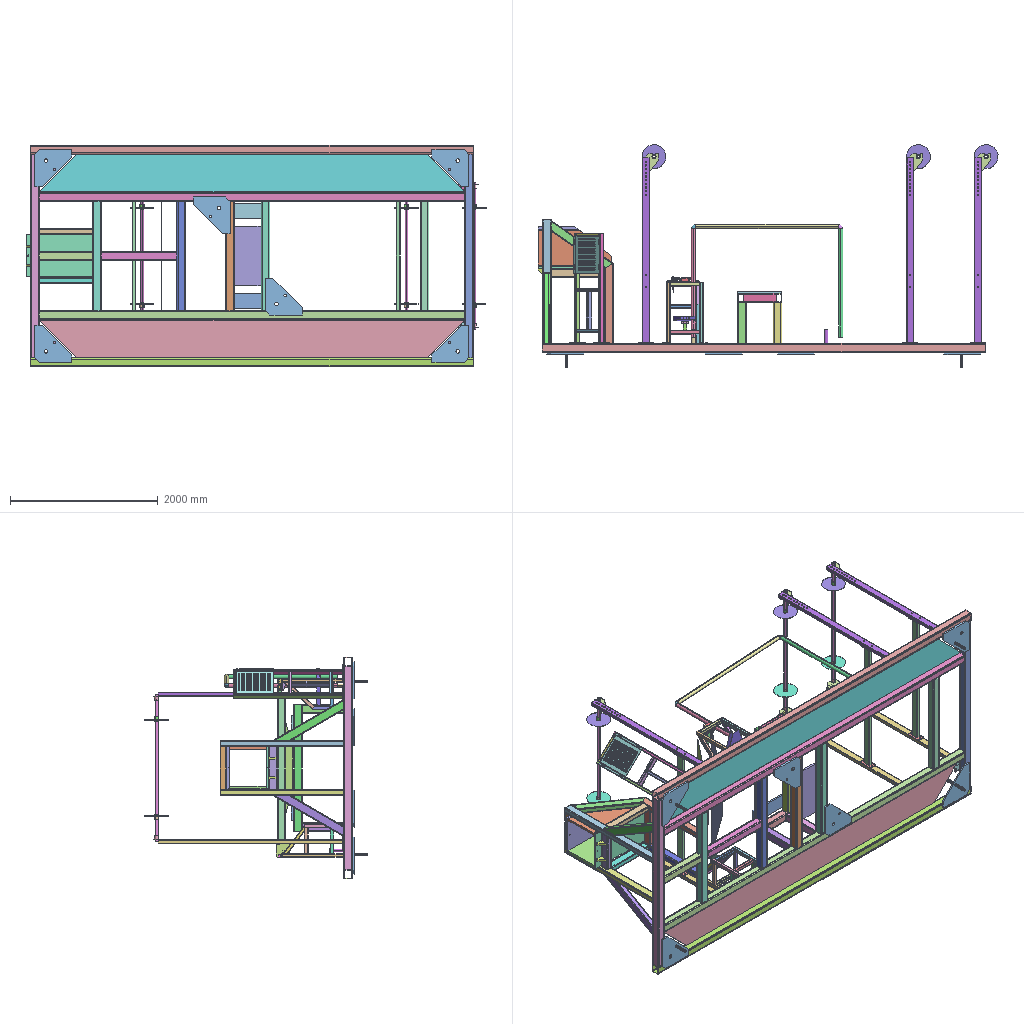Assembly | SolidWorks | 56 different items | 111 placed | box 6232 x 3016 x 3000 mm
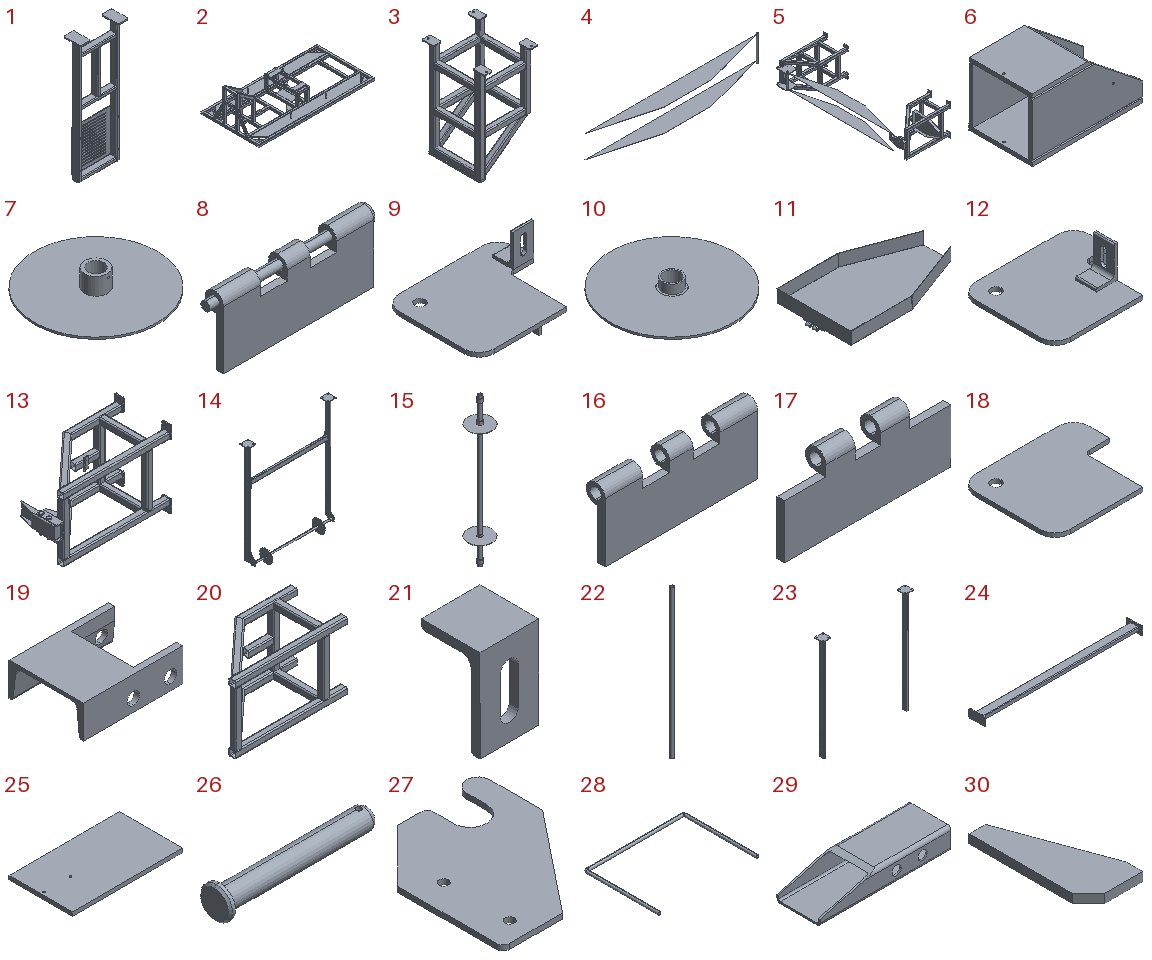Parts list (item | name | quantity | parent item | size | volume | features):
1 | (subassembly) | x1 | - | 580 x 200 x 1494 mm | 6577657 mm3 | -
2 | (subassembly) | x1 | - | 6060 x 3000 x 1995 mm | 369969133 mm3 | features ReferencePattern 10, MirrorCompFeat 5, CompositeCurve 1
3 | (subassembly) | x1 | in 5 | 470 x 550 x 847 mm | 5189358 mm3 | features ReferencePattern 3, MirrorCompFeat 2
4 | (subassembly) | x1 | in 5 | 2055 x 200.072 x 310 mm | 659869 mm3 | -
5 | (subassembly) | x1 | - | 917 x 2571 x 600 mm | 11540187 mm3 | features MirrorCompFeat 1, ReferencePattern 1
6 | (subassembly) | x1 | - | 1000 x 570 x 570 mm | 59141970 mm3 | -
7 | (subassembly) | x3 | in 15 | 325 x 325 x 74 mm | 481042 mm3 | -
8 | (subassembly) | x1 | in 13 | 92 x 10.5 x 38.25 mm | 14844 mm3 | -
9 | (subassembly) | x1 | in 5 | 220 x 184 x 134 mm | 313255 mm3 | -
10 | (subassembly) | x3 | in 15 | 325 x 325 x 74 mm | 481042 mm3 | -
11 | (subassembly) | x1 | in 5 | 510.75 x 300 x 60.5 mm | 296011 mm3 | -
12 | (subassembly) | x1 | in 5 | 220 x 184 x 134 mm | 313255 mm3 | -
13 | (subassembly) | x1 | in 5 | 891 x 440 x 600 mm | 4747445 mm3 | features ReferencePattern 3, MirrorCompFeat 2
14 | (subassembly) | x3 | - | 2200 x 372.5 x 2697 mm | 11177165 mm3 | -
15 | (subassembly) | x3 | in 14 | 325 x 325 x 2000 mm | 1601927 mm3 | features ReferencePattern 2, MirrorCompFeat 1
16 | - | x1 | in 8 | 85 x 10.5 x 38.25 mm | 12934 mm3 | features ICE 2, Chamfer 1, Cut 1, Extrusion 1
17 | - | x1 | in 11 | 85 x 10.5 x 38.25 mm | 11305 mm3 | features ICE 2, Chamfer 1, Cut 1, Extrusion 1
18 | - | x1 | in 12 | 220 x 184 x 8 mm | 271263 mm3 | features Extrusion 1
19 | - | x1 | in 13 | 160 x 120 x 53 mm | 192954 mm3 | features ICE 2, 3DProfileFeature 1, WeldMemberFeat 1, WeldmentFeature 1
20 | - | x1 | in 13 | 825 x 420 x 500 mm | 3812160 mm3 | features WeldCornerFeat 3, WeldMemberFeat 2, 3DProfileFeature 1, Cut 1, WeldmentFeature 1
21 | - | x3 | in 5, 12 | 40 x 40 x 63 mm | 20996 mm3 | features 3DProfileFeature 1, Cut 1, WeldMemberFeat 1, WeldmentFeature 1
22 | - | x3 | in 15 | 42 x 42 x 2000 mm | 502655 mm3 | features Extrusion 1
23 | - | x3 | in 14 | 2200 x 200 x 2514 mm | 6513642 mm3 | features HoleWzd 4, Fillet 2, ICE 2, MirrorSolid 2, 3DProfileFeature 1, LPattern 1, WeldMemberFeat 1, WeldmentFeature 1
24 | - | x3 | in 14 | 1950 x 200 x 100 mm | 2501619 mm3 | features Fillet 1, HoleWzd 1, ICE 1, MirrorSolid 1, WeldMemberFeat 1, WeldmentFeature 1
25 | - | x1 | in 6 | 1000 x 570 x 35 mm | 19933163 mm3 | features 3DProfileFeature 1, Extrusion 1, HoleWzd 1
26 | - | x2 | in 13 | 145 x 30 x 30 mm | 46693 mm3 | features Chamfer 1, Fillet 1, ICE 1, Revolution 1
27 | - | x6 | in 14 | 210 x 247.5 x 8 mm | 279988 mm3 | features Extrusion 1
28 | - | x1 | - | 2060 x 1530 x 60 mm | 4297442 mm3 | features 3DProfileFeature 1, WeldMemberFeat 1, WeldmentFeature 1
29 | - | x1 | in 13 | 300 x 100 x 50 mm | 358178 mm3 | features ICE 2, 3DProfileFeature 1, WeldMemberFeat 1, WeldmentFeature 1
30 | - | x2 | in 13 | 50 x 110 x 8 mm | 29800 mm3 | features Chamfer 1, Extrusion 1
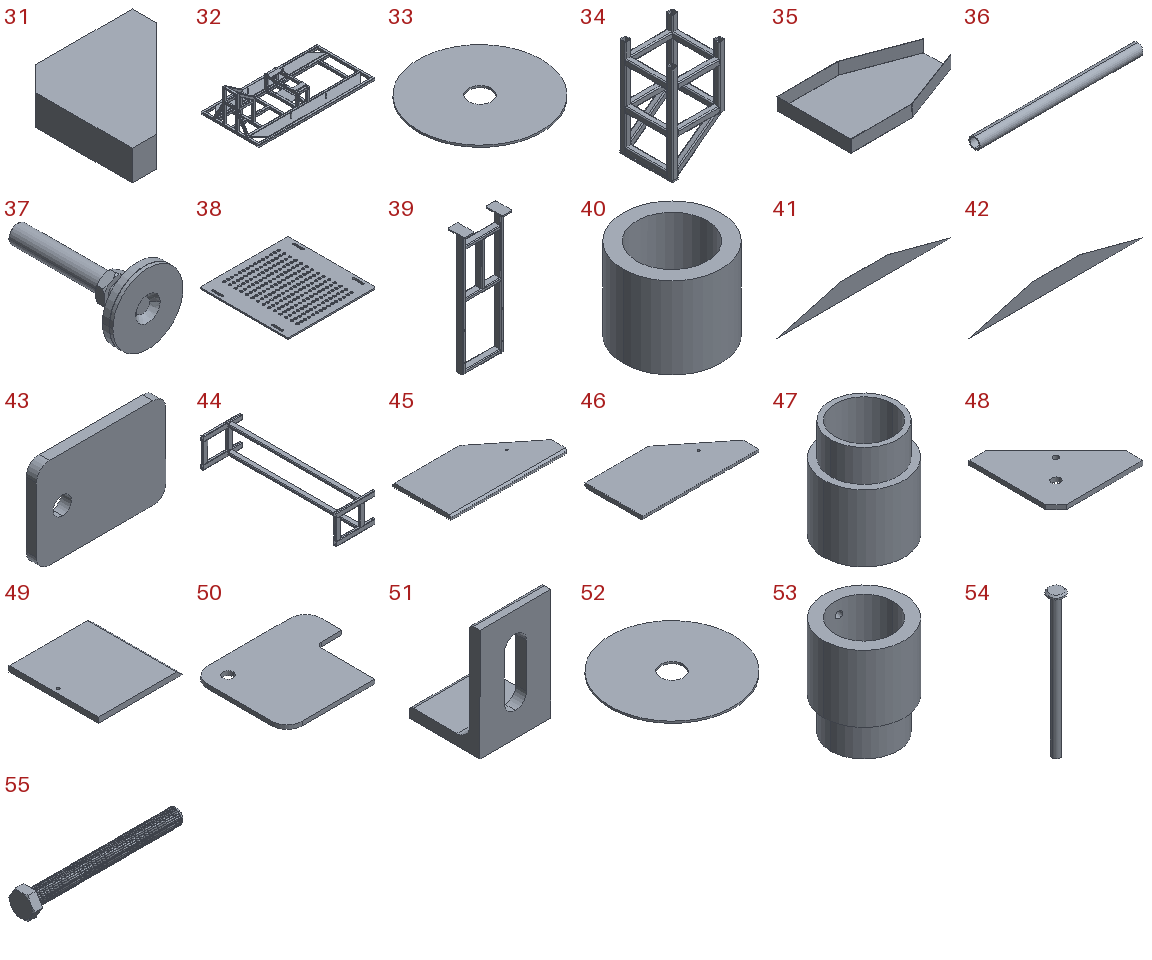31 | - | x2 | in 2 | 100 x 100 x 25 mm | 165000 mm3 | features Extrusion 1
32 | - | x1 | in 2 | 6000 x 3000 x 1795 mm | 349583429 mm3 | features WeldCornerFeat 9, ICE 4, MoveCopyBody 4, WeldMemberFeat 3, MirrorSolid 2, 3DProfileFeature 1, LPattern 1, WeldmentFeature 1
33 | - | x3 | in 7 | 325 x 325 x 5 mm | 400176 mm3 | features Extrusion 1
34 | - | x1 | in 3 | 450 x 450 x 839 mm | 4973031 mm3 | features WeldCornerFeat 2, WeldMemberFeat 2, 3DProfileFeature 1, ICE 1, WeldmentFeature 1
35 | - | x1 | in 11 | 500 x 300 x 50 mm | 284706 mm3 | features EdgeFlange 1, FlatPattern 1, SMBaseFlange 1, SheetMetal 1
36 | - | x1 | in 4 | 310 x 21.3 x 21.3 mm | 37592 mm3 | features WeldMemberFeat 1, WeldmentFeature 1
37 | - | x1 | in 2 | 200 x 371 x 200 mm | 1786955 mm3 | features ICE 2, RevCut 2, Chamfer 1, Revolution 1
38 | - | x1 | in 1 | 500 x 500 x 8 mm | 1868492 mm3 | features ICE 2, MirrorPattern 2, Extrusion 1, Fillet 1, LPattern 1
39 | - | x1 | in 1 | 580 x 200 x 1494 mm | 4709165 mm3 | features MirrorSolid 3, WeldMemberFeat 3, 3DProfileFeature 2, WeldCornerFeat 2, Cut 1, Fillet 1, ICE 1, LPattern 1, MoveCopyBody 1, WeldmentFeature 1
40 | - | x6 | in 15 | 60 x 60 x 50 mm | 68595 mm3 | features 3DProfileFeature 1, Cut 1, Extrusion 1, HoleWzd 1, ICE 1
41 | - | x1 | in 4 | 2043 x 1.2 x 200 mm | 311138 mm3 | features FlatPattern 1, SMBaseFlange 1, SheetMetal 1
42 | - | x1 | in 4 | 2043 x 1.2 x 200 mm | 311138 mm3 | features EdgeFlange 2, FlatPattern 1, SMBaseFlange 1, SheetMetal 1
43 | - | x8 | in 3, 13 | 100 x 8 x 70 mm | 54082 mm3 | features Extrusion 1, Fillet 1, ICE 1
44 | - | x1 | in 5 | 640 x 2220 x 480 mm | 6940947 mm3 | features 3DProfileFeature 1, WeldMemberFeat 1, WeldmentFeature 1
45 | - | x1 | in 6 | 1000 x 500 x 35 mm | 14402910 mm3 | features 3DProfileFeature 1, Chamfer 1, Cut 1, Extrusion 1, HoleWzd 1
46 | - | x1 | in 6 | 1000 x 500 x 35 mm | 14402910 mm3 | features 3DProfileFeature 1, Chamfer 1, Cut 1, Extrusion 1, HoleWzd 1
47 | - | x3 | in 7 | 60 x 60 x 74 mm | 80866 mm3 | features 3DProfileFeature 1, Extrusion 1, HoleWzd 1, ICE 1
48 | - | x8 | in 2 | 500 x 500 x 25 mm | 4135806 mm3 | features Chamfer 1, Cut 1, Extrusion 1, ICE 1
49 | - | x1 | in 6 | 543.75 x 570 x 35 mm | 10402988 mm3 | features 3DProfileFeature 1, Cut 1, Extrusion 1, HoleWzd 1
50 | - | x1 | in 9 | 220 x 184 x 8 mm | 271263 mm3 | features MirrorStock 1
51 | - | x2 | in 9 | 40 x 40 x 63 mm | 20996 mm3 | features MirrorStock 1
52 | - | x3 | in 10 | 325 x 325 x 5 mm | 400176 mm3 | features MirrorStock 1
53 | - | x3 | in 10 | 60 x 60 x 74 mm | 80866 mm3 | features MirrorStock 1
54 | - | x1 | in 8 | 10 x 10 x 92 mm | 1910 mm3 | features Chamfer 1, Extrusion 1, ICE 1
55 | - | x4 | in 2 | 318.7 x 53.116 x 46 mm | 228448 mm3 | features RevCut 3, Chamfer 1, Extrusion 1, Fillet 1, LPattern 1, Revolution 1, SweepThread 1
56 | Winding Yarn Glue Tank Base Plate | x1 | - | - | - | -
Mates (type | each side: item.copy, entity, surface, feature):
In the top assembly
Coincident | 32.1 face plane Gb/6728-1986 rectangular hollow section 120 X 80 X 6 (1) | 25.1 face plane Boss-Extrude1
Width | 45.1 face plane Boss-Extrude1 | assembly face | 32.1 face plane Gb/6728-1986 rectangular hollow section 120 X 80 X 6 (1) | 32.1 face plane Gb/6728-1986 rectangular hollow section 120 X 80 X 6 (1)
Coincident | 31.1 face plane Boss-Extrude1 | 25.1 face plane Boss-Extrude1
Width | 23.1 face plane Gb/6728-1986 rectangular hollow section 100 X 50 X 4 (1) | 23.1 face plane Gb/6728-1986 rectangular hollow section 100 X 50 X 4 (1) | 32.1 face plane Gb/t 6728—2002 square hollow section 120×8 (1) | 32.1 face plane Gb/t 6728—2002 square hollow section 120×8 (1)
Coincident | 32.1 face plane Mirror6 | 23.1 face plane Mirror1
Width | 23.2 face plane Gb/6728-1986 rectangular hollow section 100 X 50 X 4 (1) | 23.2 face plane Gb/6728-1986 rectangular hollow section 100 X 50 X 4 (1) | 32.1 face plane Gb/t 6728—2002 square hollow section 120×8 (1) | 32.1 face plane Gb/t 6728—2002 square hollow section 120×8 (1)
Coincident | 32.1 face plane Mirror6 | 23.2 face plane Mirror1
Coincident | 32.1 face plane Mirror6 | 23.3 face plane Mirror1
Width | 23.3 face plane Gb/6728-1986 rectangular hollow section 100 X 50 X 4 (1) | 23.3 face plane Gb/6728-1986 rectangular hollow section 100 X 50 X 4 (1) | 32.1 face plane Gb/t 6728—2002 square hollow section 120×8 (1) | 32.1 face plane Gb/t 6728—2002 square hollow section 120×8 (1)
Coincident | 32.1 face plane Gb/6728-1986 rectangular hollow section 120 X 80 X 6 (1) | 45.1 face plane Boss-Extrude1
DistanceDim | assembly face | 32.1 face plane Mirror6
Coincident | 32.1 face plane Mirror6 | 43.1 face plane Boss-Extrude1
Width | 34.1 face plane Gb/6728-1986 square hollow section 050 X 50 X 4 (1) | 20.1 face plane Gb/6728-1986 square hollow section 050 X 50 X 4 (1) | 32.1 face plane Gb/t 6728—2002 square hollow section 120×8 (1) | 32.1 face plane Gb/t 6728—2002 square hollow section 120×8 (1)
Coincident | 32.1 face plane Mirror6 | 39.1 face plane Boss-Extrude1
Concentric | 32.1 face cylinder Mirror6 | 28.1 face cylinder Gb/t6728-2002 round tube 060 X 5 (1)
In subassembly 6
Coincident | 25.2 face plane Boss-Extrude1 | 45.2 face plane Boss-Extrude1 | 3 times
Coincident | 25.2 face plane Boss-Extrude1 | 49.1 face plane Boss-Extrude1
Coincident | 25.2 face plane Boss-Extrude1 | 46.1 face plane Boss-Extrude1 | 3 times
In subassembly 14
Width | 24.1 face plane Mirror2 | 24.1 face plane Boss-Extrude1 | 23.4 face plane Gb/6728-1986 rectangular hollow section 100 X 50 X 4 (1) | 23.4 face plane Gb/6728-1986 rectangular hollow section 100 X 50 X 4 (1) | 2 times
Concentric | 23.4 face cylinder M16 Clearance Hole3 | 27.1 face cylinder Boss-Extrude1
Concentric | 23.4 face cylinder LPattern1 | 27.1 face cylinder Boss-Extrude1
Coincident | 23.4 face plane Gb/6728-1986 rectangular hollow section 100 X 50 X 4 (1) | 27.1 face plane Boss-Extrude1
Coincident | 23.4 face plane Gb/6728-1986 rectangular hollow section 100 X 50 X 4 (1) | 27.2 face plane Boss-Extrude1
Concentric | 23.4 face cylinder M16 Clearance Hole3 | 27.2 face cylinder Boss-Extrude1
Concentric | 23.4 face cylinder LPattern1 | 27.2 face cylinder Boss-Extrude1
Concentric | 27.1 face cylinder Boss-Extrude1 | 22.1 face cylinder Boss-Extrude1
Width | 22.1 face plane Boss-Extrude1 | 22.1 face plane Boss-Extrude1 | 27.1 face plane Boss-Extrude1 | 27.2 face plane Boss-Extrude1
Parallel | 23.4 face plane Gb/6728-1986 rectangular hollow section 100 X 50 X 4 (1) | 24.1 face plane Gb/6728-1986 rectangular hollow section 100 X 50 X 4 (1)
Coincident | 23.4 face plane Gb/6728-1986 rectangular hollow section 100 X 50 X 4 (1) | 24.1 face plane Mirror2
Concentric | 23.4 face cylinder M16 Clearance Hole4 | 24.1 face cylinder M16 Clearance Hole2
In subassembly 15
Concentric | 22.2 face cylinder Boss-Extrude1 | 47.1 face cylinder Boss-Extrude1
DistanceDim | 47.1 face plane Boss-Extrude1 | 22.2 face plane Boss-Extrude1
Concentric | 22.2 face cylinder Boss-Extrude1 | 40.1 face cylinder Boss-Extrude1
DistanceDim | 40.1 face plane Boss-Extrude1 | 53.1 face plane Stop Piece_Mirror
In subassembly 7
Concentric | 33.1 face cylinder Boss-Extrude1 | 47.2 face cylinder Boss-Extrude2
Coincident | 33.1 face plane Boss-Extrude1 | 47.2 face plane Boss-Extrude1
In subassembly 1
Width | 38.1 face plane Boss-Extrude1 | 38.1 face plane Boss-Extrude1 | 39.2 face plane Gb/6728-1986 rectangular hollow section 80 X 40 X 4 (1) | 39.2 face plane Gb/6728-1986 rectangular hollow section 80 X 40 X 4 (1)
Coincident | 39.2 face plane Gb/6728-1986 rectangular hollow section 80 X 40 X 4 (1) | 38.1 face plane Boss-Extrude1 | 2 times
In subassembly 5
Coincident | 43.2 face plane Boss-Extrude1 | 43.3 face plane Boss-Extrude1
Coincident | 34.2 face plane Gb/6728-1986 square hollow section 050 X 50 X 4 (1) | 20.2 face plane Gb/6728-1986 square hollow section 050 X 50 X 4 (1)
Coincident | 34.2 face plane Gb/6728-1986 square hollow section 050 X 50 X 4 (1) | 20.2 face plane Gb/6728-1986 square hollow section 050 X 50 X 4 (12)
Coincident | 34.2 face plane Boss-Extrude1 | 18.1 face plane Boss-Extrude1 | 2 times
Concentric | 36.1 face cylinder Gb/t6728-2002 round tube 021.3 X 2 (1) | 18.1 face cylinder Boss-Extrude1 | 2 times
Coincident | 18.1 face plane Boss-Extrude1 | 21.1 face plane Hot-rolled unequal angle GB∕T 706-2008 63 X 40 X 6 (1)
Coincident | 21.2 face plane Hot-rolled unequal angle GB∕T 706-2008 63 X 40 X 6 (1) | 21.1 face plane Hot-rolled unequal angle GB∕T 706-2008 63 X 40 X 6 (1)
Coincident | 34.2 face plane Boss-Extrude1 | 21.1 face plane Hot-rolled unequal angle GB∕T 706-2008 63 X 40 X 6 (1)
DistanceDim | 21.2 face plane Hot-rolled unequal angle GB∕T 706-2008 63 X 40 X 6 (1) | 34.2 face plane Boss-Extrude1
Width | 18.1 face plane Boss-Extrude1 | 50.1 face plane Fixing Plate_Mirror | 36.1 face plane Gb/t6728-2002 round tube 021.3 X 2 (1) | 36.1 face plane Gb/t6728-2002 round tube 021.3 X 2 (1)
Concentric | 54.1 face cylinder Boss-Extrude1 | 17.1 face cylinder Cut-Extrude3
Coincident | 16.1 face plane Cut-Extrude2 | 17.1 face plane Cut-Extrude2
DistanceDim | 20.2 face plane Gb/6728-1986 square hollow section 050 X 50 X 4 (1) | 34.2 face plane Gb/6728-1986 square hollow section 050 X 50 X 4 (1)
In subassembly 12
Coincident | 18.2 face plane Boss-Extrude1 | 21.3 face plane Hot-rolled unequal angle GB∕T 706-2008 63 X 40 X 6 (1) | 3 times
Coincident | 18.2 face plane Boss-Extrude1 | 21.1 face plane Hot-rolled unequal angle GB∕T 706-2008 63 X 40 X 6 (1) | 2 times
DistanceDim | 18.2 face plane Boss-Extrude1 | 21.1 face plane Hot-rolled unequal angle GB∕T 706-2008 63 X 40 X 6 (1)
In subassembly 11
Coincident | 35.1 face plane Base-Flange1 | 17.2 face plane Boss-Extrude1
Width | 17.2 face plane Boss-Extrude1 | 17.2 face plane Boss-Extrude1 | 35.1 face plane Edge-Flange1 | 35.1 face plane Edge-Flange1
Coincident | 35.1 face plane Edge-Flange1 | 17.2 face plane Cut-Extrude2
In subassembly 3
Coincident | 34.3 face plane Gb/6728-1986 square hollow section 050 X 50 X 4 (1) | 43.4 face plane Boss-Extrude1 | 2 times
Width | 43.4 face plane Boss-Extrude1 | 43.4 face plane Boss-Extrude1 | 34.3 face plane Gb/6728-1986 square hollow section 050 X 50 X 4 (1) | 34.3 face plane Gb/6728-1986 square hollow section 050 X 50 X 4 (1)
In subassembly 13
Coincident | 20.3 face plane Gb/6728-1986 square hollow section 050 X 50 X 4 (1) | 43.4 face plane Boss-Extrude1 | 2 times
Coincident | 20.3 face plane Gb/6728-1986 square hollow section 050 X 50 X 4 (1) | 16.2 face plane Boss-Extrude1
Width | 16.2 face plane Boss-Extrude1 | 16.2 face plane Boss-Extrude1 | 20.3 face plane Gb/6728-1986 square hollow section 050 X 50 X 4 (1) | 20.3 face plane Gb/6728-1986 square hollow section 050 X 50 X 4 (1)
DistanceDim | 16.2 face plane Boss-Extrude1 | 20.3 face plane Gb/6728-1986 square hollow section 050 X 50 X 4 (1)
Coincident | 20.3 face plane Gb/6728-1986 square hollow section 050 X 50 X 4 (1) | 19.1 face plane C-channel 12(1) | 2 times
Width | 19.1 face plane C-channel 12(1) | 19.1 face plane C-channel 12(1) | 20.3 face plane Gb/6728-1986 square hollow section 050 X 50 X 4 (1) | 20.3 face plane Gb/6728-1986 square hollow section 050 X 50 X 4 (1)
Coincident | 19.1 face plane C-channel 12(1) | 30.1 face plane Boss-Extrude1 | 3 times
Coincident | 19.1 face plane C-channel 12(1) | 30.2 face plane Boss-Extrude1 | 3 times
Concentric | 19.1 face cylinder Cut-Extrude2 | 29.1 face cylinder Cut-Extrude1 | 2 times
Width | 29.1 face plane Rectangular tube 100 X 50 X 4 (1) | 29.1 face plane Rectangular tube 100 X 50 X 4 (1) | 19.1 face plane C-channel 12(1) | 19.1 face plane C-channel 12(1)
Concentric | 19.1 face cylinder Cut-Extrude2 | 26.1 face cylinder Base-Revolve
Coincident | 19.1 face plane C-channel 12(1) | 26.1 face plane Base-Revolve
Concentric | 19.1 face cylinder Cut-Extrude2 | 26.2 face cylinder Base-Revolve
Coincident | 19.1 face plane C-channel 12(1) | 26.2 face plane Base-Revolve
Width | 43.4 face plane Boss-Extrude1 | 43.4 face plane Boss-Extrude1 | 20.3 face plane Gb/6728-1986 square hollow section 050 X 50 X 4 (1) | 20.3 face plane Gb/6728-1986 square hollow section 050 X 50 X 4 (1)
In subassembly 8
InPlace | 16.3 face plane Boss-Extrude1 | 54.2 plane
In subassembly 9
Coincident | 50.2 face plane Fixing Plate_Mirror | 51.1 face plane Fixing Angle Iron_Mirror | 3 times
Coincident | 50.2 face plane Fixing Plate_Mirror | 51.2 face plane Fixing Angle Iron_Mirror | 2 times
DistanceDim | 50.2 face plane Fixing Plate_Mirror | 51.2 face plane Fixing Angle Iron_Mirror
In subassembly 2
Coincident | 32.2 face plane Gb/t 6728—2002 square hollow section 120×8 (1) | 48.1 face plane Boss-Extrude1
DistanceDim | 48.1 face plane Boss-Extrude1 | 32.2 face plane Gb/t 6728—2002 square hollow section 120×8 (1)
DistanceDim | 32.2 face plane Gb/t 6728—2002 square hollow section 120×8 (1) | 48.1 face plane Boss-Extrude1
Concentric | 48.1 face cylinder Cut-Extrude1 | 37.1 face
DistanceDim | 37.1 face | 48.1 face plane Boss-Extrude1
DistanceDim | 31.2 face plane Boss-Extrude1 | 32.2 face plane Gb/6728-1986 rectangular hollow section 120 X 80 X 6 (1)
Coincident | 32.2 face plane Gb/6728-1986 rectangular hollow section 120 X 80 X 6 (1) | 31.2 face plane Boss-Extrude1 | 2 times
DistanceDim | 48.2 face plane Boss-Extrude1 | 32.2 face plane Gb/t 6728—2002 square hollow section 120×8 (1)
Concentric | 37.2 face | 48.3 face cylinder Cut-Extrude1
DistanceDim | 37.2 face | 48.3 face plane Boss-Extrude1
DistanceDim | 48.4 face plane Boss-Extrude1 | 32.2 face plane Gb/t 6728—2002 square hollow section 120×8 (1)
Concentric | 37.3 face | 48.5 face cylinder Cut-Extrude1
DistanceDim | 48.5 face plane Boss-Extrude1 | 37.3 face
Coincident | 32.2 face plane Gb/t 6728—2002 square hollow section 120×8 (1) | 48.3 face plane Boss-Extrude1
DistanceDim | 48.3 face plane Boss-Extrude1 | 32.2 face plane Gb/t 6728—2002 square hollow section 120×8 (1) | 2 times
DistanceDim | 48.5 face plane Boss-Extrude1 | 32.2 face plane Gb/t 6728—2002 square hollow section 120×8 (1) | 2 times
Coincident | 32.2 face plane Gb/t 6728—2002 square hollow section 120×8 (1) | 48.5 face plane Boss-Extrude1
Concentric | 48.1 face cylinder Cut-Extrude2 | 55.1 edge
DistanceDim | 55.1 face plane Base-Extrude | 48.1 face plane Boss-Extrude1